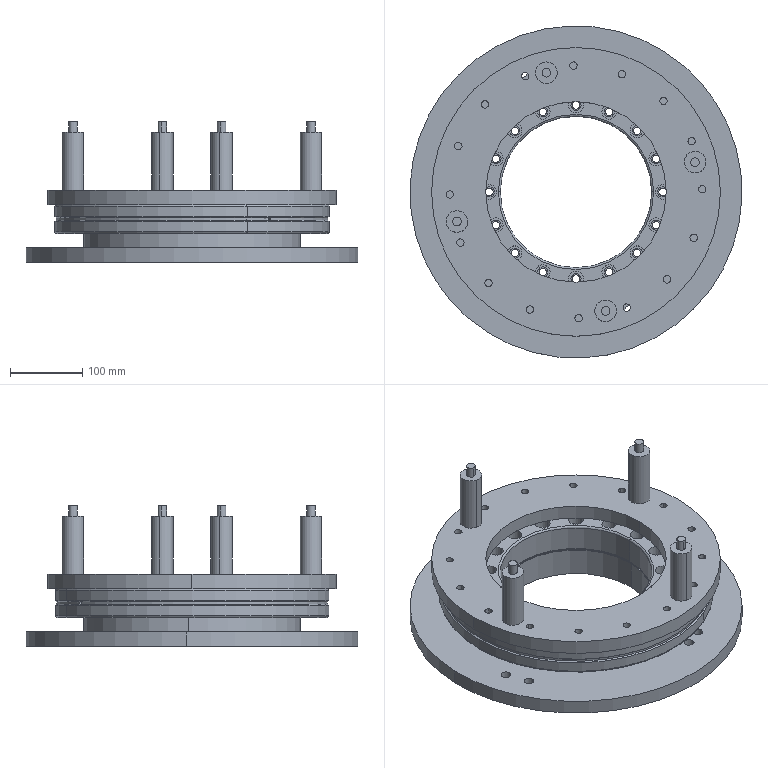Part | SolidWorks | features InContextFeatHolder 6, ReferencePattern 3, LocalCirPattern 1 | 40 solids | 652 faces | box 460 x 460 x 195 mm | volume 7776901 mm3 | cylinder 357 | torus 138 | plane 129 | cone 28 | commonest cylinder face diameters 12 x66 10.2 x64 14 x64 20 x64 13.5 x16 8.5 x8